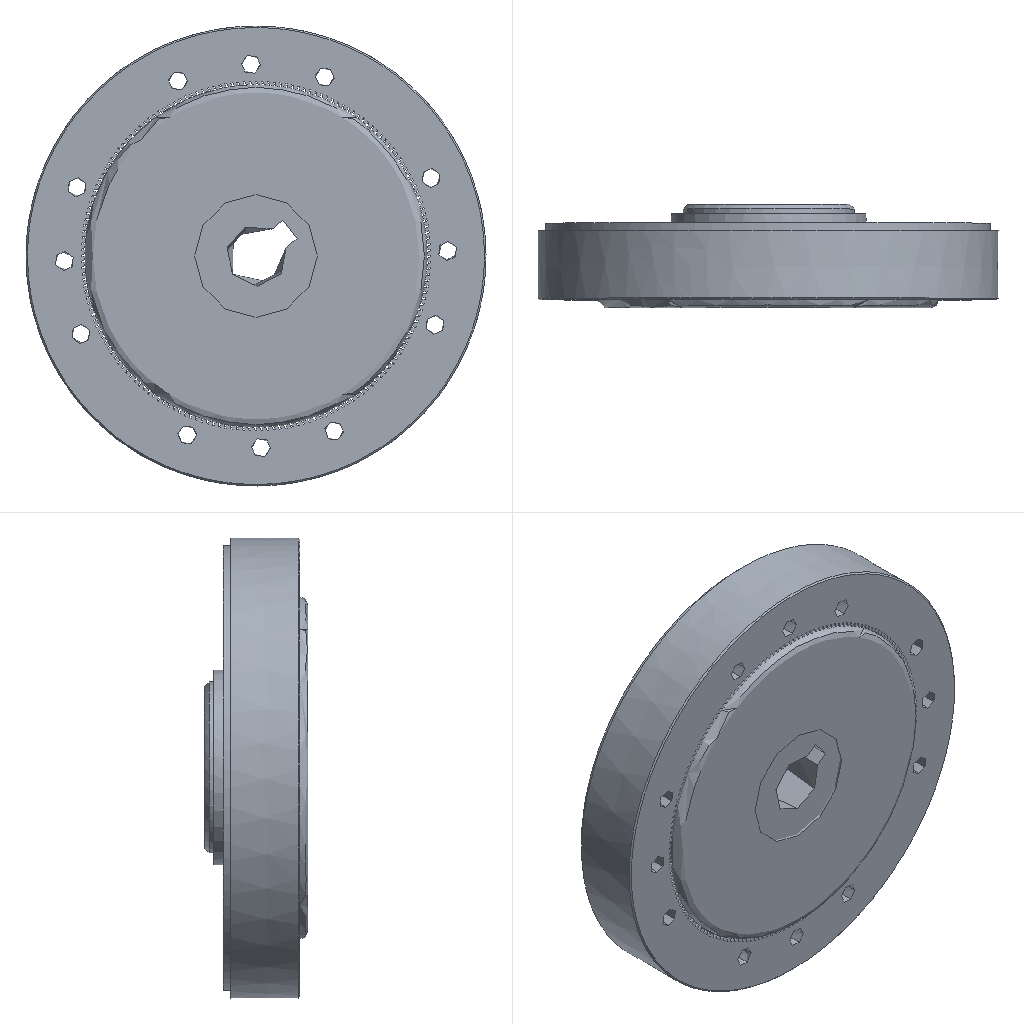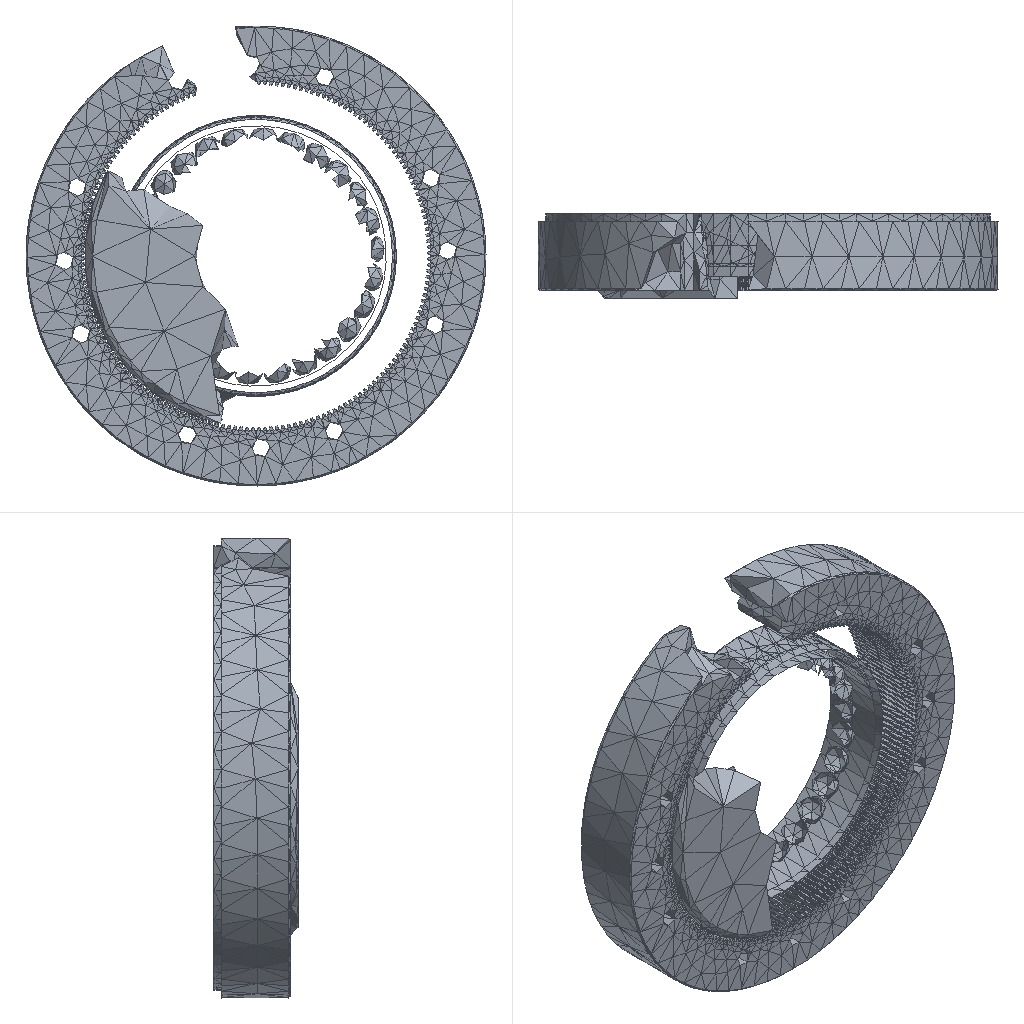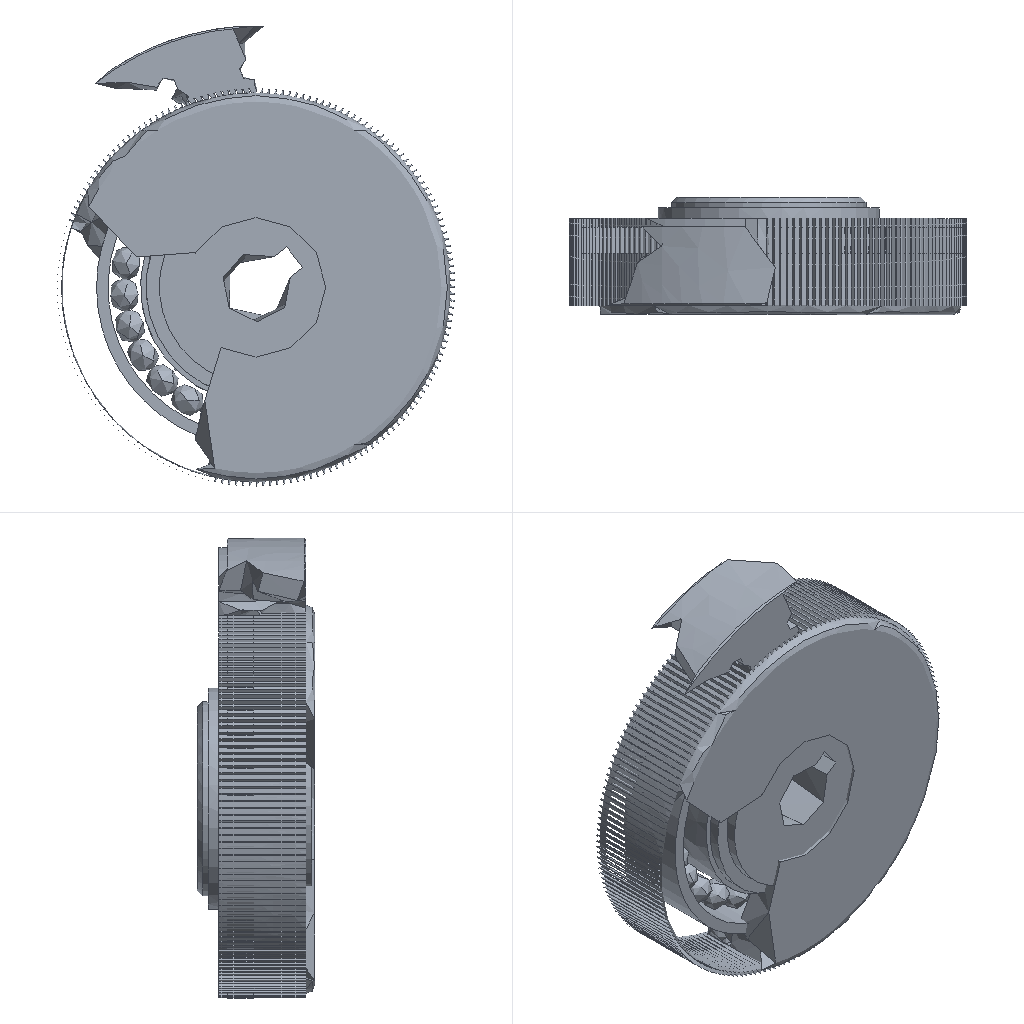Simulation study | ansys workbench
Set-up summary:
category,name,step,type,value,unit,region
solver,ansys_workbench
units,SI m-kg-s (Pa),,stated,"/units,MKS"
analysis,LS1,,static
load_step,LS1,LS1,static,nsubst=1; time=1
mesh,nodes,,,99605
mesh,elements,,,83282
element_type,SOLID187,,,52324
element_type,CONTA174,,,16650
element_type,TARGE170,,,14208
element_type,SOLID186,,,100
material,40CrMnSiA,,E,2.09e+11,Pa
material,40CrMnSiA,,nu,0.29
material,40CrMnSiA,,density,7850,kg m^-3
material,GCr15,,E,2.1e+11,Pa
material,GCr15,,nu,0.3
material,GCr15,,density,7810,kg m^-3
material,45?,,E,2.09e+11,Pa
material,45?,,nu,0.269
material,45?,,density,7850,kg m^-3
load,,LS1,moment,"2.5 [dir=(0, 1, 0) n=3]",,all
bc,Fixed Supports,model,fixed,[dofs=ALL],,_FIXEDSU
contact,Contact Region,,bonded (always),element=CONTA174
contact,Contact Region 2,,bonded (always),element=CONTA174
contact,Contact Region 3,,bonded (always),element=CONTA174
contact,contact 4,,bonded (always),element=CONTA174
named_set,_CM53_FIXEDSU,,node,906
named_set,_CM55_FIXEDSU,,node,352
named_set,_FIXEDSU,,node,1258
Ansys APDL input file, long lists of numbers shortened:
/batch
/config,noeldb,1     ! force off writing results to database
*get,_wallstrt,active,,time,wall
! ANSYS input file written by Workbench version 2022 R1
! File used for geometry attach:
/title,wbnew--____ (B5)
! ****** Begin Custom Load Command Snippet ******
/COM, ACT Extensions:
/COM,     LSDYNA, 2021.1
/COM,
! ****** End   Custom Load Command Snippet ******
*DIM,_wb_ProjectScratch_dir,string,248
_wb_ProjectScratch_dir(1) = ''
*DIM,_wb_SolverFiles_dir,string,248
_wb_SolverFiles_dir(1) = ''
*DIM,_wb_userfiles_dir,string,248
_wb_userfiles_dir(1) = ''
/com,--- Data in consistent MKS units. See Solving Units in the help system for more information.
/units,MKS
/nopr
/wb,file,start              !  signify a WB generated input file
/prep7
! Turn off shape checking because checks already performed inside WB mesher.
! See help system for more information.
SHPP,OFF,,NOWARN
/nolist
etcon,set             ! allow ANSYS to choose best KEYOP's for 180x elements, resets any applicable keyopt to MAPDL defaults
/com,*********** Nodes for the whole assembly ***********
nblock,3,,109564
(1i9,3e20.9e3)
        1     1.577421328E-02     1.100000000E-02     9.277079036E-03
! (99603 more lines like these left out)
-1
/com,*********** Nodes for all Remote Points ***********
nblock,3
(1i9,3e20.9e3)
    99605     6.296733752E-03     6.303704855E-03     1.046924175E-03
-1
/wb,elem,start            !  set before creation of elements
/com,*********** Elements for Body 1 "__|__3" ***********
et,1,187
eblock,19,solid,,20391
(19i9)
        1        1        1        1        0        0        0        0       10        0     8432    16767    21977    22585    22104    29006    53741    29008    29007
! (40781 more lines like these left out)
-1
/com,*********** Elements for Body 2 "____|____2[1]" ***********
et,2,186
keyo,2,2,1          ! set full integration on SOLID186
eblock,19,solid,,100
(19i9)
        2        2        2        2        0        0        0        0       20        0        1      151      244      243      152      177      267      266      176
! (199 more lines like these left out)
-1
/com,*********** Elements for Body 3 "____|__-__4" ***********
et,3,187
eblock,19,solid,,8331
(19i9)
        3        3        3        3        0        0        0        0       10        0      101     2949     3202     3350     3334    15114    15901    15117    15116
! (16661 more lines like these left out)
-1
/com,*********** Elements for Body 4 "__|__1" ***********
et,4,187
eblock,19,solid,,23602
(19i9)
        4        4        4        4        0        0        0        0       10        0    28823    56915    61985    59505    60691    74751    88157    74749    74750
! (47203 more lines like these left out)
-1
/wb,elem,end               !  done creating elements
/com,*********** Send User Defined Coordinate System(s) ***********
csys,0
toffst,273.15,  ! Temperature offset from absolute zero
/com,*********** Set Reference Temperature ***********
tref,22.
/wb,mat,start              !  starting to send materials
/com,*********** Send Materials ***********
MP,EX,1,209000000000,	! Pa
MP,NUXY,1,0.29,
MP,DENS,1,7850,	! kg m^-3
MP,EX,2,210000000000,	! Pa
MP,NUXY,2,0.3,
MP,DENS,2,7810,	! kg m^-3
MP,EX,3,210000000000,	! Pa
MP,NUXY,3,0.3,
MP,DENS,3,7810,	! kg m^-3
MP,EX,4,209000000000,	! Pa
MP,NUXY,4,0.269,
MP,DENS,4,7850,	! kg m^-3
/wb,mat,end                !  done sending materials
!************************* Model Summary ********************
!__|__3,	40CrMnSiA,	matid,	1
!____|____2[1],	GCr15,	matid,	2
!____|__-__4,	GCr15,	matid,	3
!__|__1,	45钢,	matid,	4
!************************* End Model Summary ********************
! get the diagonal of the bounding box. Needed later for other things
*get,_xmin,node,,mnloc,x
*get,_ymin,node,,mnloc,y
*get,_zmin,node,,mnloc,z
*get,_xmax,node,,mxloc,x
*get,_ymax,node,,mxloc,y
*get,_zmax,node,,mxloc,z
_ASMDIAG=(_xmax-_xmin)*(_xmax-_xmin)+(_ymax-_ymin)*(_ymax-_ymin)+(_zmax-_zmin)*(_zmax-_zmin)
_ASMDIAG=SQRT(_ASMDIAG)
/wb,contact,start          !  starting to send contact
/com,*********** Create Contact "接触区域" ***********
/com,            Real Constant Set For Above Contact Is 6 & 5
*set,tid,6
*set,cid,5
r,tid
r,cid
et,tid,170
et,cid,174
eblock,10,,,380
(15i9)
    79758        6        6        6        0    16023    16037    17692    17692    22598    22720    17692    22599
! (379 more lines like these left out)
-1
eblock,10,,,380
(15i9)
    80138        5        5        5        0    16023    16037    17692    17692    22598    22720    17692    22599
! (379 more lines like these left out)
-1
eblock,10,,,96
(15i9)
    80518        5        6        5        0      142       93       69       68      513      465      462      463
! (95 more lines like these left out)
-1
eblock,10,,,96
(15i9)
    80614        6        5        6        0      142       93       69       68      513      465      462      463
! (95 more lines like these left out)
-1
keyo,cid,8,2               ! auto create asymmetric contact (from Program Controlled setting)
keyo,cid,10,0              ! adjust contact stiffness each NR iteration (from Program Controlled setting)
keyo,cid,12,5              ! bonded always
keyo,cid,18,1              ! small sliding turned on by application
keyo,cid,2,0               ! augmented Lagrange (from Program Controlled setting)
keyo,cid,4,0               ! on Gauss point (from Program Controlled setting)
keyo,cid,9,1               ! ignore initial gaps/penetration
keyo,cid,7,0               ! No Prediction
rmod,tid,3,10.      ! FKN
rmod,tid,5,0.       ! ICONT
rmod,tid,6,0.       ! PINB
rmod,tid,10,0.      ! CNOF
rmod,tid,12,0.      ! FKT
rmod,tid,36,38      ! WB DSID
rmod,cid,3,10.      ! FKN
rmod,cid,5,0.       ! ICONT
rmod,cid,6,0.       ! PINB
rmod,cid,10,0.      ! CNOF
rmod,cid,12,0.      ! FKT
rmod,cid,36,38      ! WB DSID
/com,*********** Create Contact "接触区域 2" ***********
/com,            Real Constant Set For Above Contact Is 8 & 7
*set,tid,8
*set,cid,7
r,tid
r,cid
et,tid,170
et,cid,174
eblock,10,,,6452
(15i9)
    80710        8        8        8        0    16180    16181    20944    20944    24092    24105    20944    24096
! (6451 more lines like these left out)
-1
eblock,10,,,6452
(15i9)
    87162        7        7        7        0    16180    16181    20944    20944    24092    24105    20944    24096
! (6451 more lines like these left out)
-1
eblock,10,,,6480
(15i9)
    93614        7        8        7        0    55931    55929    57670    57670    68680    68684    57670    68695
! (6479 more lines like these left out)
-1
eblock,10,,,6480
(15i9)
   100094        8        7        8        0    55931    55929    57670    57670    68680    68684    57670    68695
! (6479 more lines like these left out)
-1
keyo,cid,8,2               ! auto create asymmetric contact (from Program Controlled setting)
keyo,cid,10,0              ! adjust contact stiffness each NR iteration (from Program Controlled setting)
keyo,cid,12,5              ! bonded always
keyo,cid,18,1              ! small sliding turned on by application
keyo,cid,2,0               ! augmented Lagrange (from Program Controlled setting)
keyo,cid,4,0               ! on Gauss point (from Program Controlled setting)
keyo,cid,9,1               ! ignore initial gaps/penetration
keyo,cid,7,0               ! No Prediction
rmod,tid,3,10.      ! FKN
rmod,tid,5,0.       ! ICONT
rmod,tid,6,0.       ! PINB
rmod,tid,10,0.      ! CNOF
rmod,tid,12,0.      ! FKT
rmod,tid,36,41      ! WB DSID
rmod,cid,3,10.      ! FKN
rmod,cid,5,0.       ! ICONT
rmod,cid,6,0.       ! PINB
rmod,cid,10,0.      ! CNOF
rmod,cid,12,0.      ! FKT
rmod,cid,36,41      ! WB DSID
/com,*********** Create Contact "接触区域 3" ***********
/com,            Real Constant Set For Above Contact Is 10 & 9
*set,tid,10
*set,cid,9
r,tid
r,cid
et,tid,170
et,cid,174
eblock,10,,,88
(15i9)
   106574       10       10       10        0      187      143       67       66      642      461      458      460
! (87 more lines like these left out)
-1
eblock,10,,,88
(15i9)
   106662        9        9        9        0      187      143       67       66      642      461      458      460
! (87 more lines like these left out)
-1
eblock,10,,,712
(15i9)
   106750        9       10        9        0     1124     1122     2618     2618     5202     5207     2618     5223
! (711 more lines like these left out)
-1
eblock,10,,,712
(15i9)
   107462       10        9       10        0     1124     1122     2618     2618     5202     5207     2618     5223
! (711 more lines like these left out)
-1
keyo,cid,8,2               ! auto create asymmetric contact (from Program Controlled setting)
keyo,cid,10,0              ! adjust contact stiffness each NR iteration (from Program Controlled setting)
keyo,cid,12,5              ! bonded always
keyo,cid,18,1              ! small sliding turned on by application
keyo,cid,2,0               ! augmented Lagrange (from Program Controlled setting)
keyo,cid,4,0               ! on Gauss point (from Program Controlled setting)
keyo,cid,9,1               ! ignore initial gaps/penetration
keyo,cid,7,0               ! No Prediction
rmod,tid,3,10.      ! FKN
rmod,tid,5,0.       ! ICONT
rmod,tid,6,0.       ! PINB
rmod,tid,10,0.      ! CNOF
rmod,tid,12,0.      ! FKT
rmod,tid,36,44      ! WB DSID
rmod,cid,3,10.      ! FKN
rmod,cid,5,0.       ! ICONT
rmod,cid,6,0.       ! PINB
rmod,cid,10,0.      ! CNOF
rmod,cid,12,0.      ! FKT
rmod,cid,36,44      ! WB DSID
nsel,all
esel,all
/wb,contact,end            !  done creating contacts
/golist
/wb,load,start             !  starting to send loads
CMBLOCK,_CM53_FIXEDSU,NODE,      906
(8i10)
      1390      1391      1392      1393      1394      1395      1396      1397
! (113 more lines like these left out)
CMBLOCK,_CM55_FIXEDSU,NODE,      352
(8i10)
        24        25        26        27        28        29        30        31
! (43 more lines like these left out)
/com,*********** Fixed Supports ***********
CMBLOCK,_FIXEDSU,NODE,     1258
(8i10)
        24        25        26        27        28        29        30        31
! (157 more lines like these left out)
cmsel,s,_FIXEDSU
d,all,all
nsel,all
/com,*********** Create Remote Point "内部远程点" ***********
! -------- Remote Point Used by "力矩" --------
*set,tid,12
*set,cid,11
et,cid,174
et,tid,170
keyo,tid,2,1               ! Don't fix the pilot node
keyo,tid,4,111111
keyo,cid,12,5              ! Bonded Contact
keyo,cid,4,1               ! Deformable RBE3 style load
keyo,cid,2,2               ! MPC style contact
eblock,10,,,2442
(15i9)
   108174       11       11       11        0    16180    16181    20944    20944    24092    24105    20944    24096
! (2441 more lines like these left out)
-1
*set,_npilot,99605
_npilot58=_npilot
type,tid
mat ,cid
real,cid
tshape,pilo
en,110616,_npilot
tshape
/com,*********** Construct Moment Using Remote Attachment ***********
/gst,on,on
fini
*get,_numnode,node,0,count
*get,_numelem,elem,0,count
*get, _MAXELEMNUM, elem, 0, NUM, MAX
*get, _MAXNODENUM, node, 0, NUM, MAX
*get, _MAXELEMTYPE, etyp, 0, NUM, MAX
*get, _MAXREALCONST, real, 0, NUM, MAX
/go
/wb,load,end               !  done creating loads
/com,--- Number of total nodes = %_numnode%
/com,--- Number of contact elements = 30858
/com,--- Number of spring elements = 0
/com,--- Number of bearing elements = 0
/com,--- Number of solid elements = 52424
/com,--- Number of condensed parts = 0
/com,--- Number of total elements = %_numelem%
*get,_wallbsol,active,,time,wall
/com,****************************************************************************
/com,*************************    SOLUTION       ********************************
/com,****************************************************************************
/solu
antype,0                   ! static analysis
_thickRatio=0.75    ! Ratio of thick parts in the model
eqsl,pcg,1e-8,,,,,,1
cntr,print,1               ! print out contact info and also make no initial contact an error
nldiag,cont,iter           ! print out contact info each equilibrium iteration
rescontrol,linear,last           ! Turn on restart files due to future eigen analysis intent
/com,****************************************************
/com,******************* SOLVE FOR LS 1 OF 1 ****************
nsel,s,node,,99605
f,all,mx,0.
f,all,my,2.5
f,all,mz,0.
nsel,all
/nopr
/gopr
nsub,1,1,1
time,1.
outres,erase
outres,all,none
outres,nsol,all,
outres,rsol,all
outres,eangl,all
outres,etmp,all
outres,veng,all
outres,strs,all,
outres,epel,all,
outres,eppl,all,
outres,cont,all,
! *********** WB SOLVE COMMAND ***********
! check interactive state
*get,ANSINTER_,active,,int
*if,ANSINTER_,ne,0,then
/eof
*endif
solve
/com *************** Write FE CONNECTORS *********
CEWRITE,file,ce,,INTE
/com,****************************************************
/com,*************** FINISHED SOLVE FOR LS 1 *************
*get,_wallasol,active,,time,wall
/nopr
*get,_numnode,node,0,count
*get,_numelem,elem,0,count
*get, _MAXELEMNUM, elem, 0, NUM, MAX
*get, _MAXNODENUM, node, 0, NUM, MAX,,,INTERNAL
*get, _MAXELEMTYPE, etyp, 0, NUM, MAX
*get, _MAXREALCONST, real, 0, NUM, MAX
/gopr
*get,_PCGITER,active,,solu,cgiter
/post1
xmlo,ENCODING,ISO-8859-1
xmlo,parm
/xml,parm,xml
fini
/gopr
*get,_walldone,active,,time,wall
_preptime=(_wallbsol-_wallstrt)*3600
_solvtime=(_wallasol-_wallbsol)*3600
_posttime=(_walldone-_wallasol)*3600
_totaltim=(_walldone-_wallstrt)*3600
*get,_dlbratio,active,0,solu,dlbr
*get,_combtime,active,0,solu,comb
*get,_ssmode,active,0,solu,ssmm
*get,_ndofs,active,0,solu,ndof
/com,--- Total number of nodes = %_numnode%
/com,--- Total number of elements = %_numelem%
/com,--- Element load balance ratio = %_dlbratio%
/com,--- Time to combine distributed files = %_combtime%
/com,--- Sparse memory mode = %_ssmode%
/com,--- Number of DOF = %_ndofs%
/wb,file,end               ! done with WB generated input
Results summary:
result,analyses[0].index,,,1
result,analyses[0].system,,,SYS
result,analyses[0].deck,,,deck.dat
result,analyses[0].solve_status,,,completed
result,analyses[0].analysis_type,,,static
result,analyses[0].physics,,,mechanical
result,analyses[0].unit_system,,,"MKS: m, kg, N, s, V, A, degC"
result,analyses[0].n_sets,,,1
result,analyses[0].load_steps[0].set,set=1,,1
result,analyses[0].load_steps[0].time_or_freq,set=1,,1
result,analyses[0].load_steps[0].max_displacement_magnitude,set=1,,4.18297e-08
result,analyses[0].load_steps[0].max_von_mises_nodal,set=1,,2.79034e+07
result,analyses[0].load_steps[0].reaction_force_sum_xyz[1],set=1,,2.78667e-07
result,analyses[0].load_steps[0].reaction_force_sum_xyz[2],set=1,,-3.49391e-07
result,analyses[0].load_steps[0].reaction_force_sum_xyz[3],set=1,,1.29142e-06